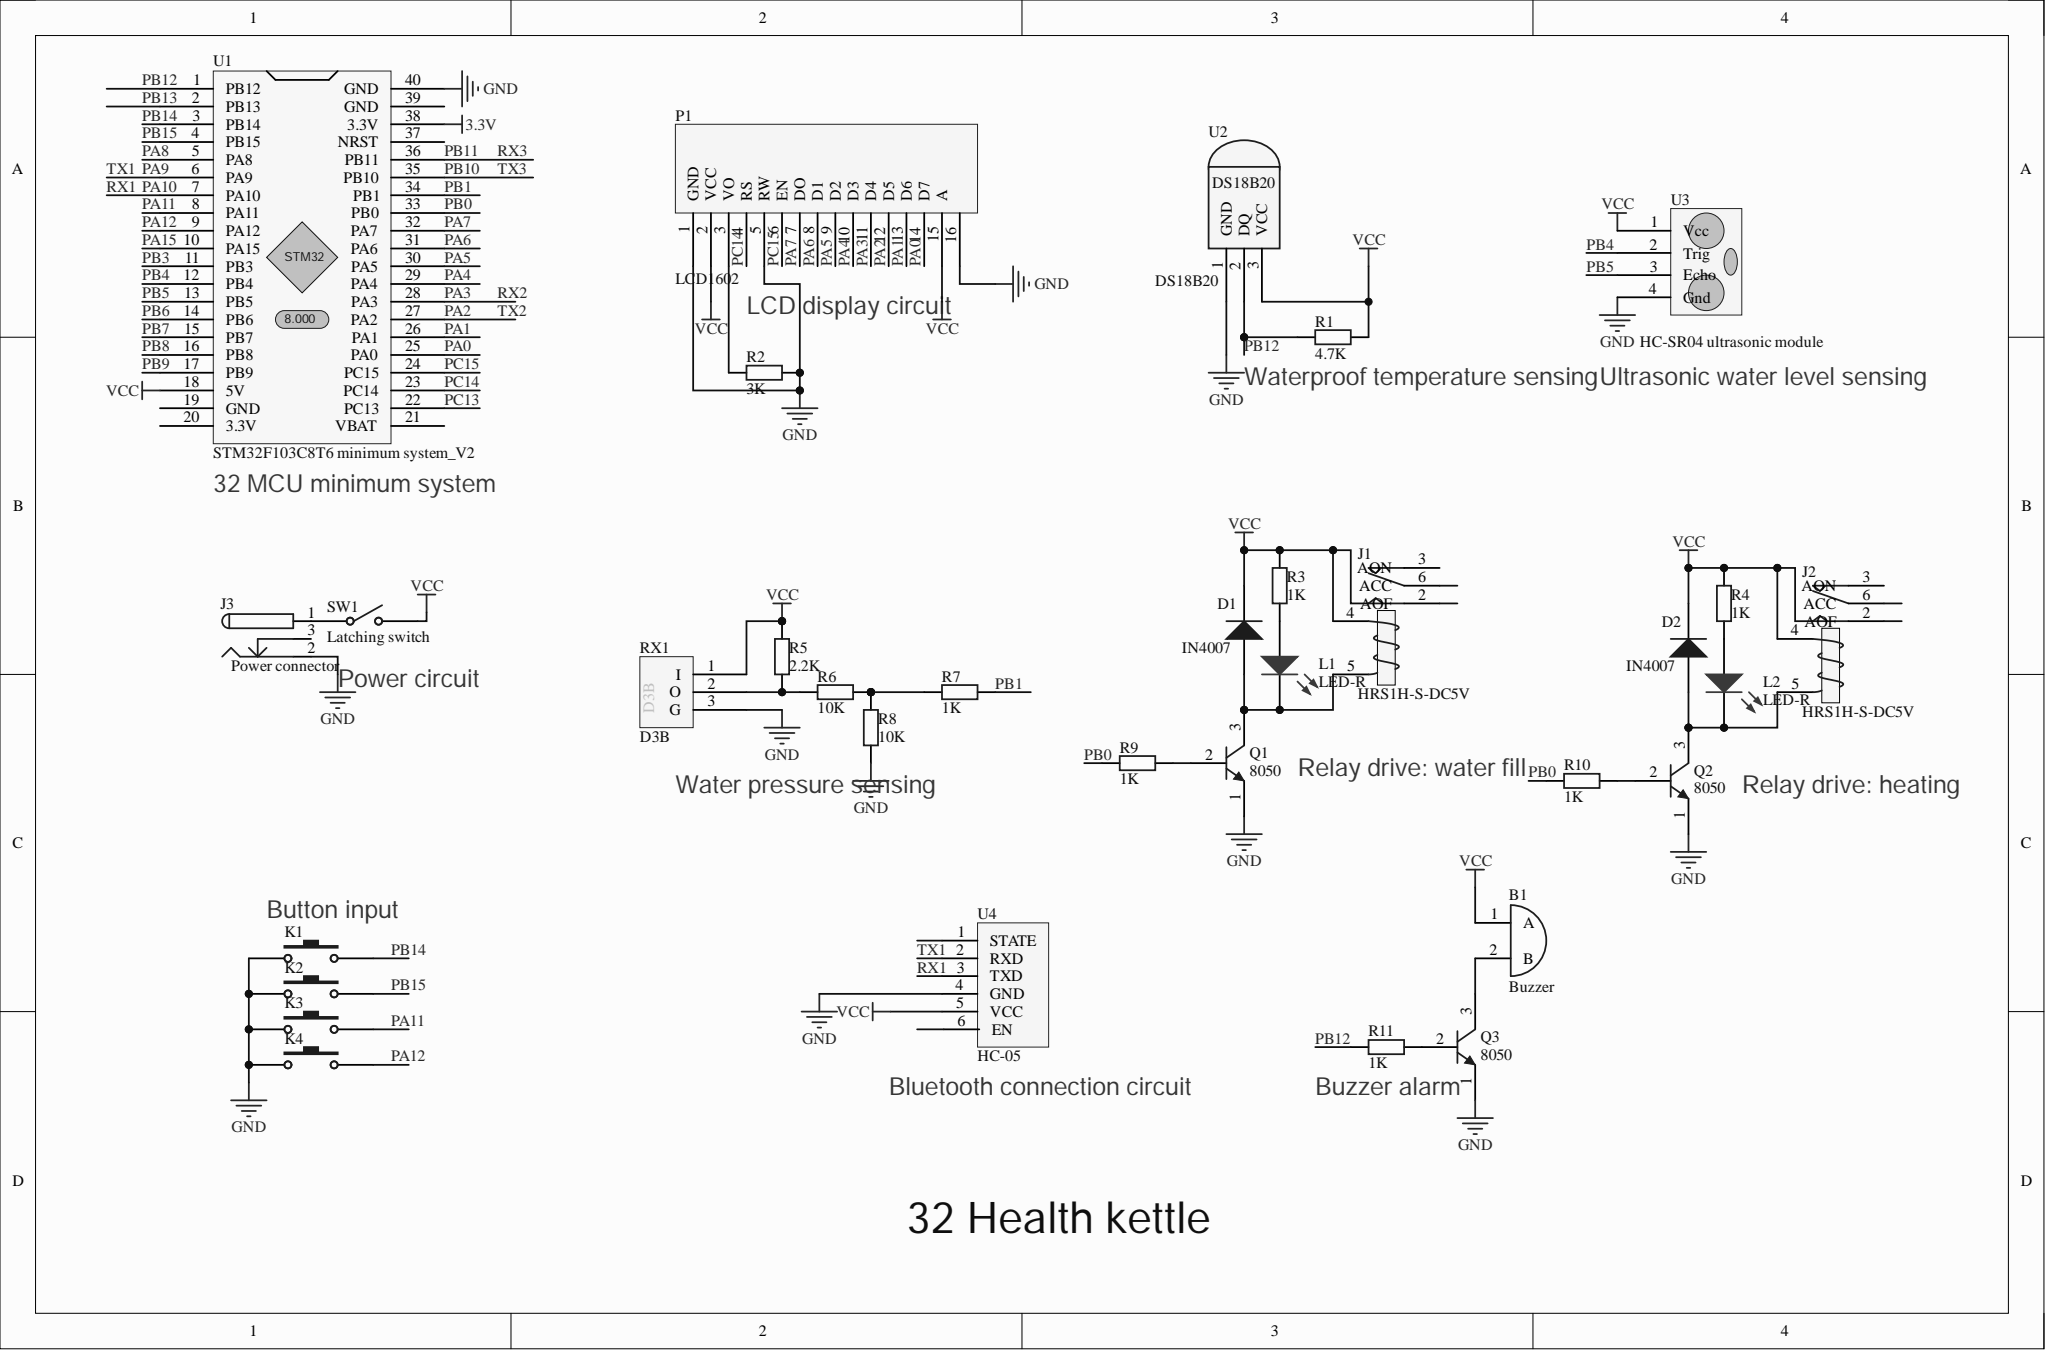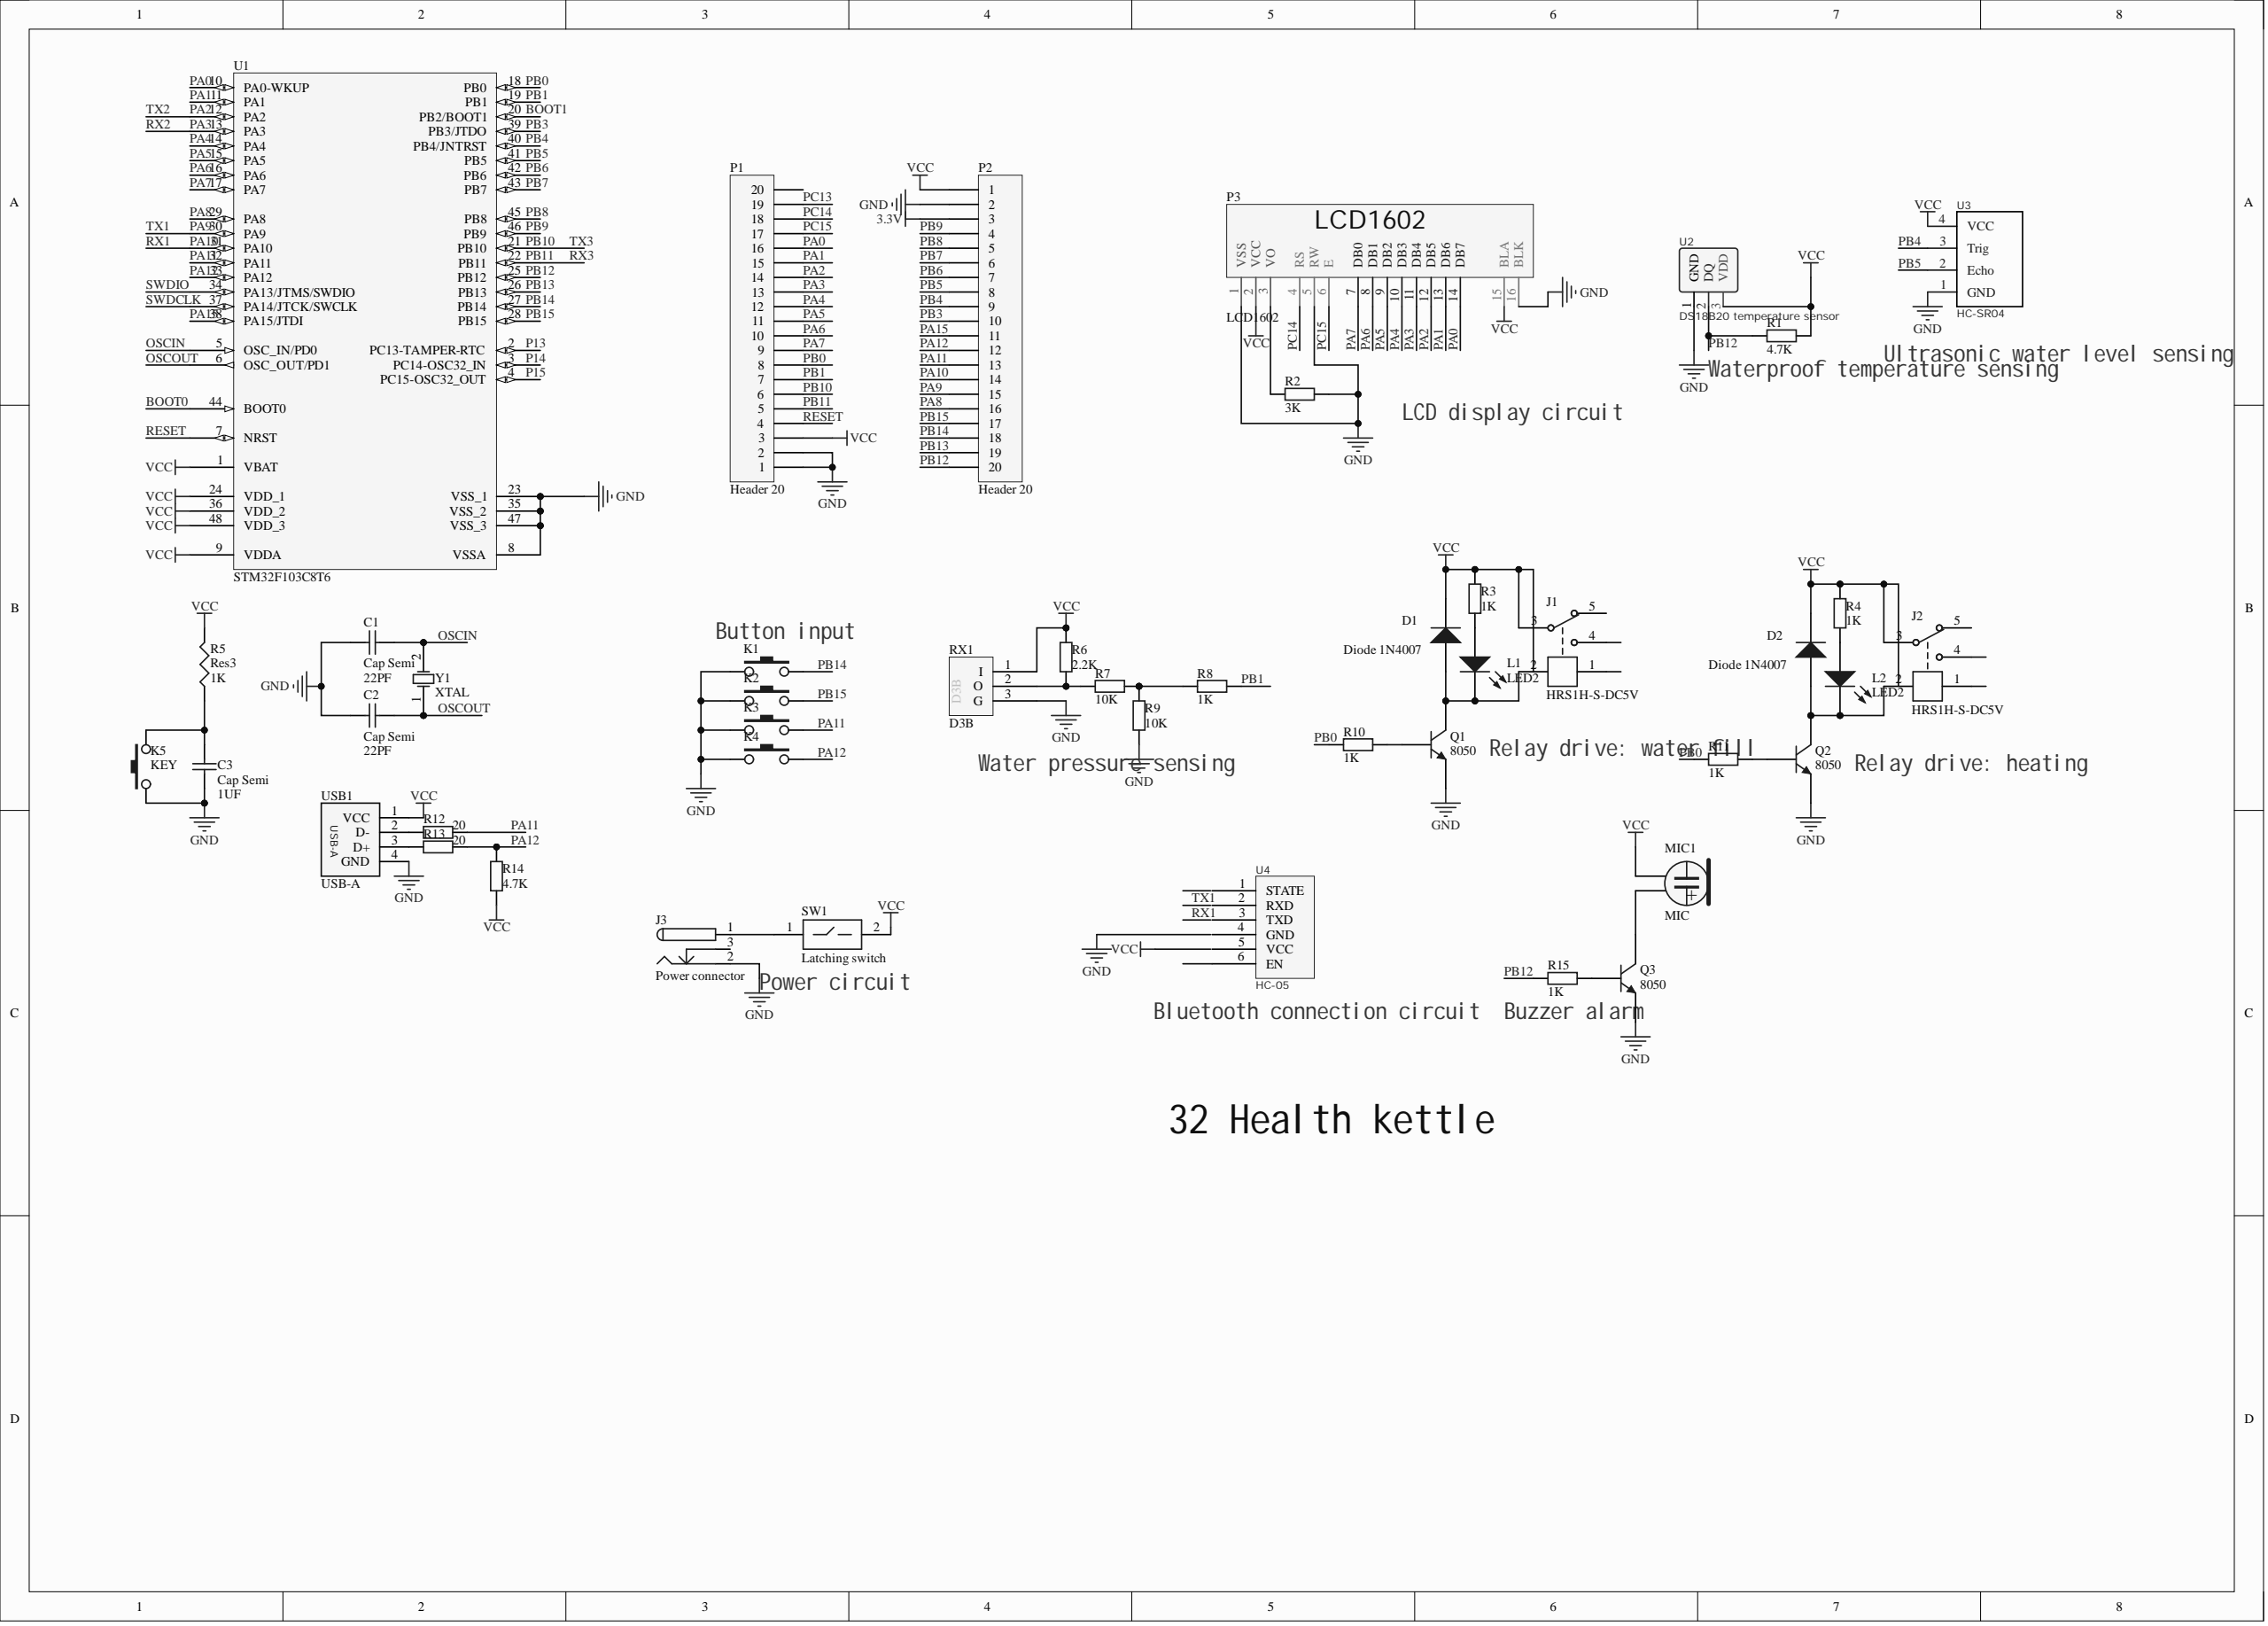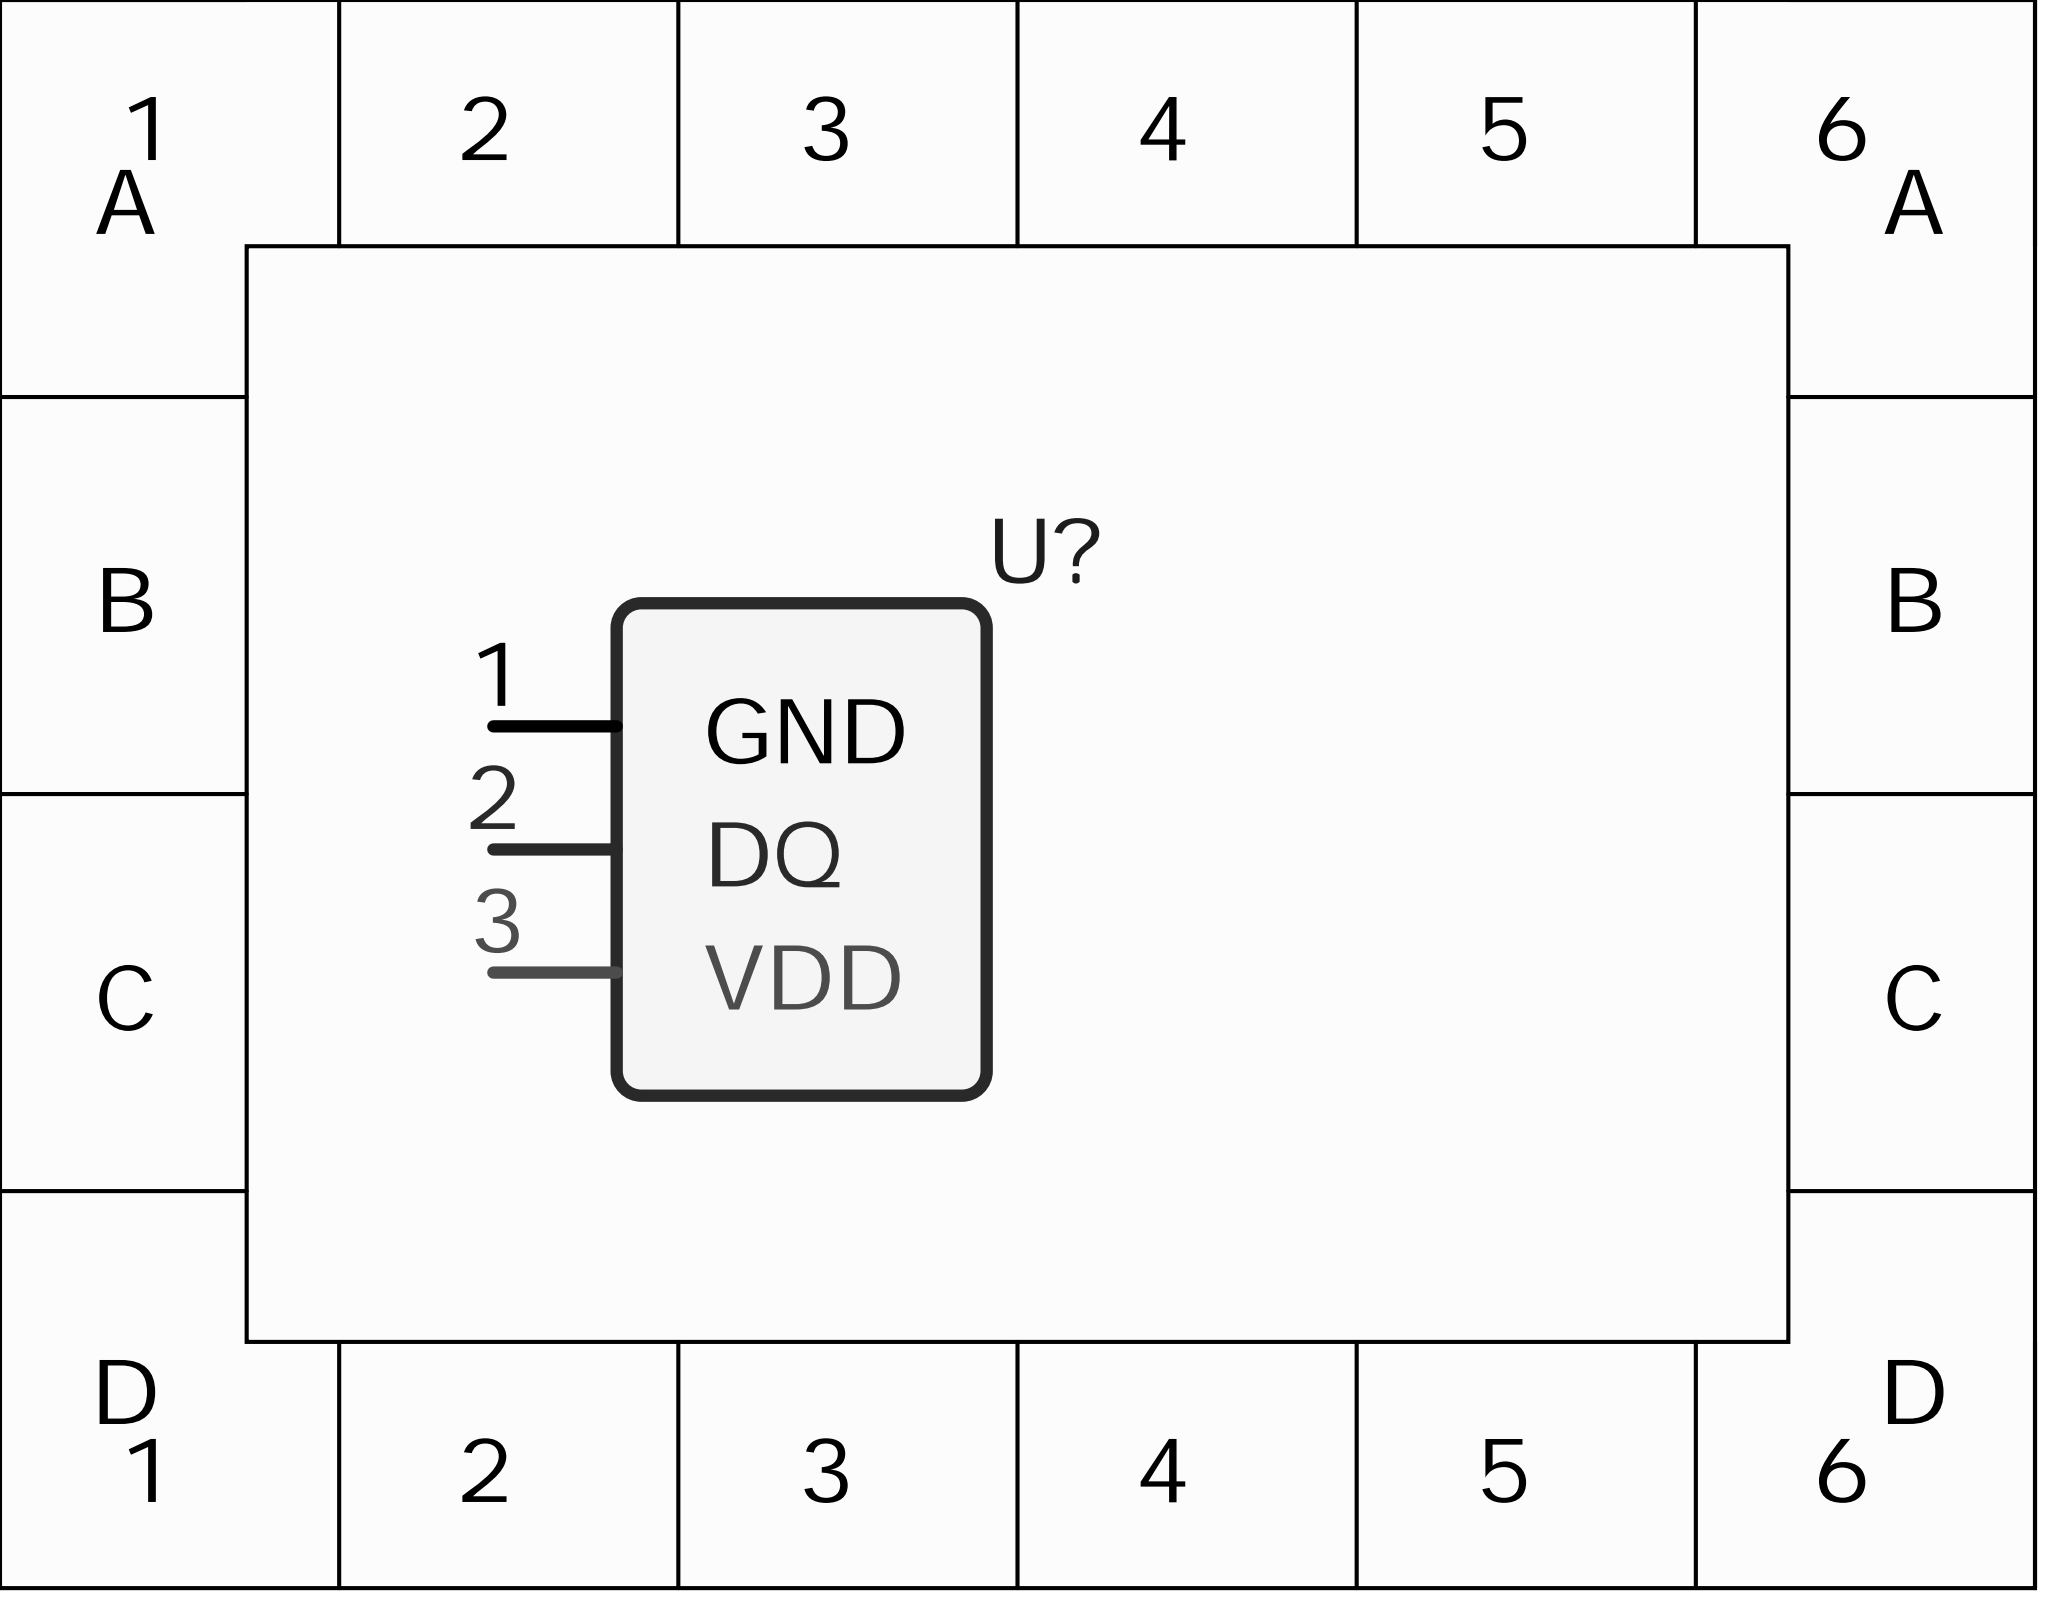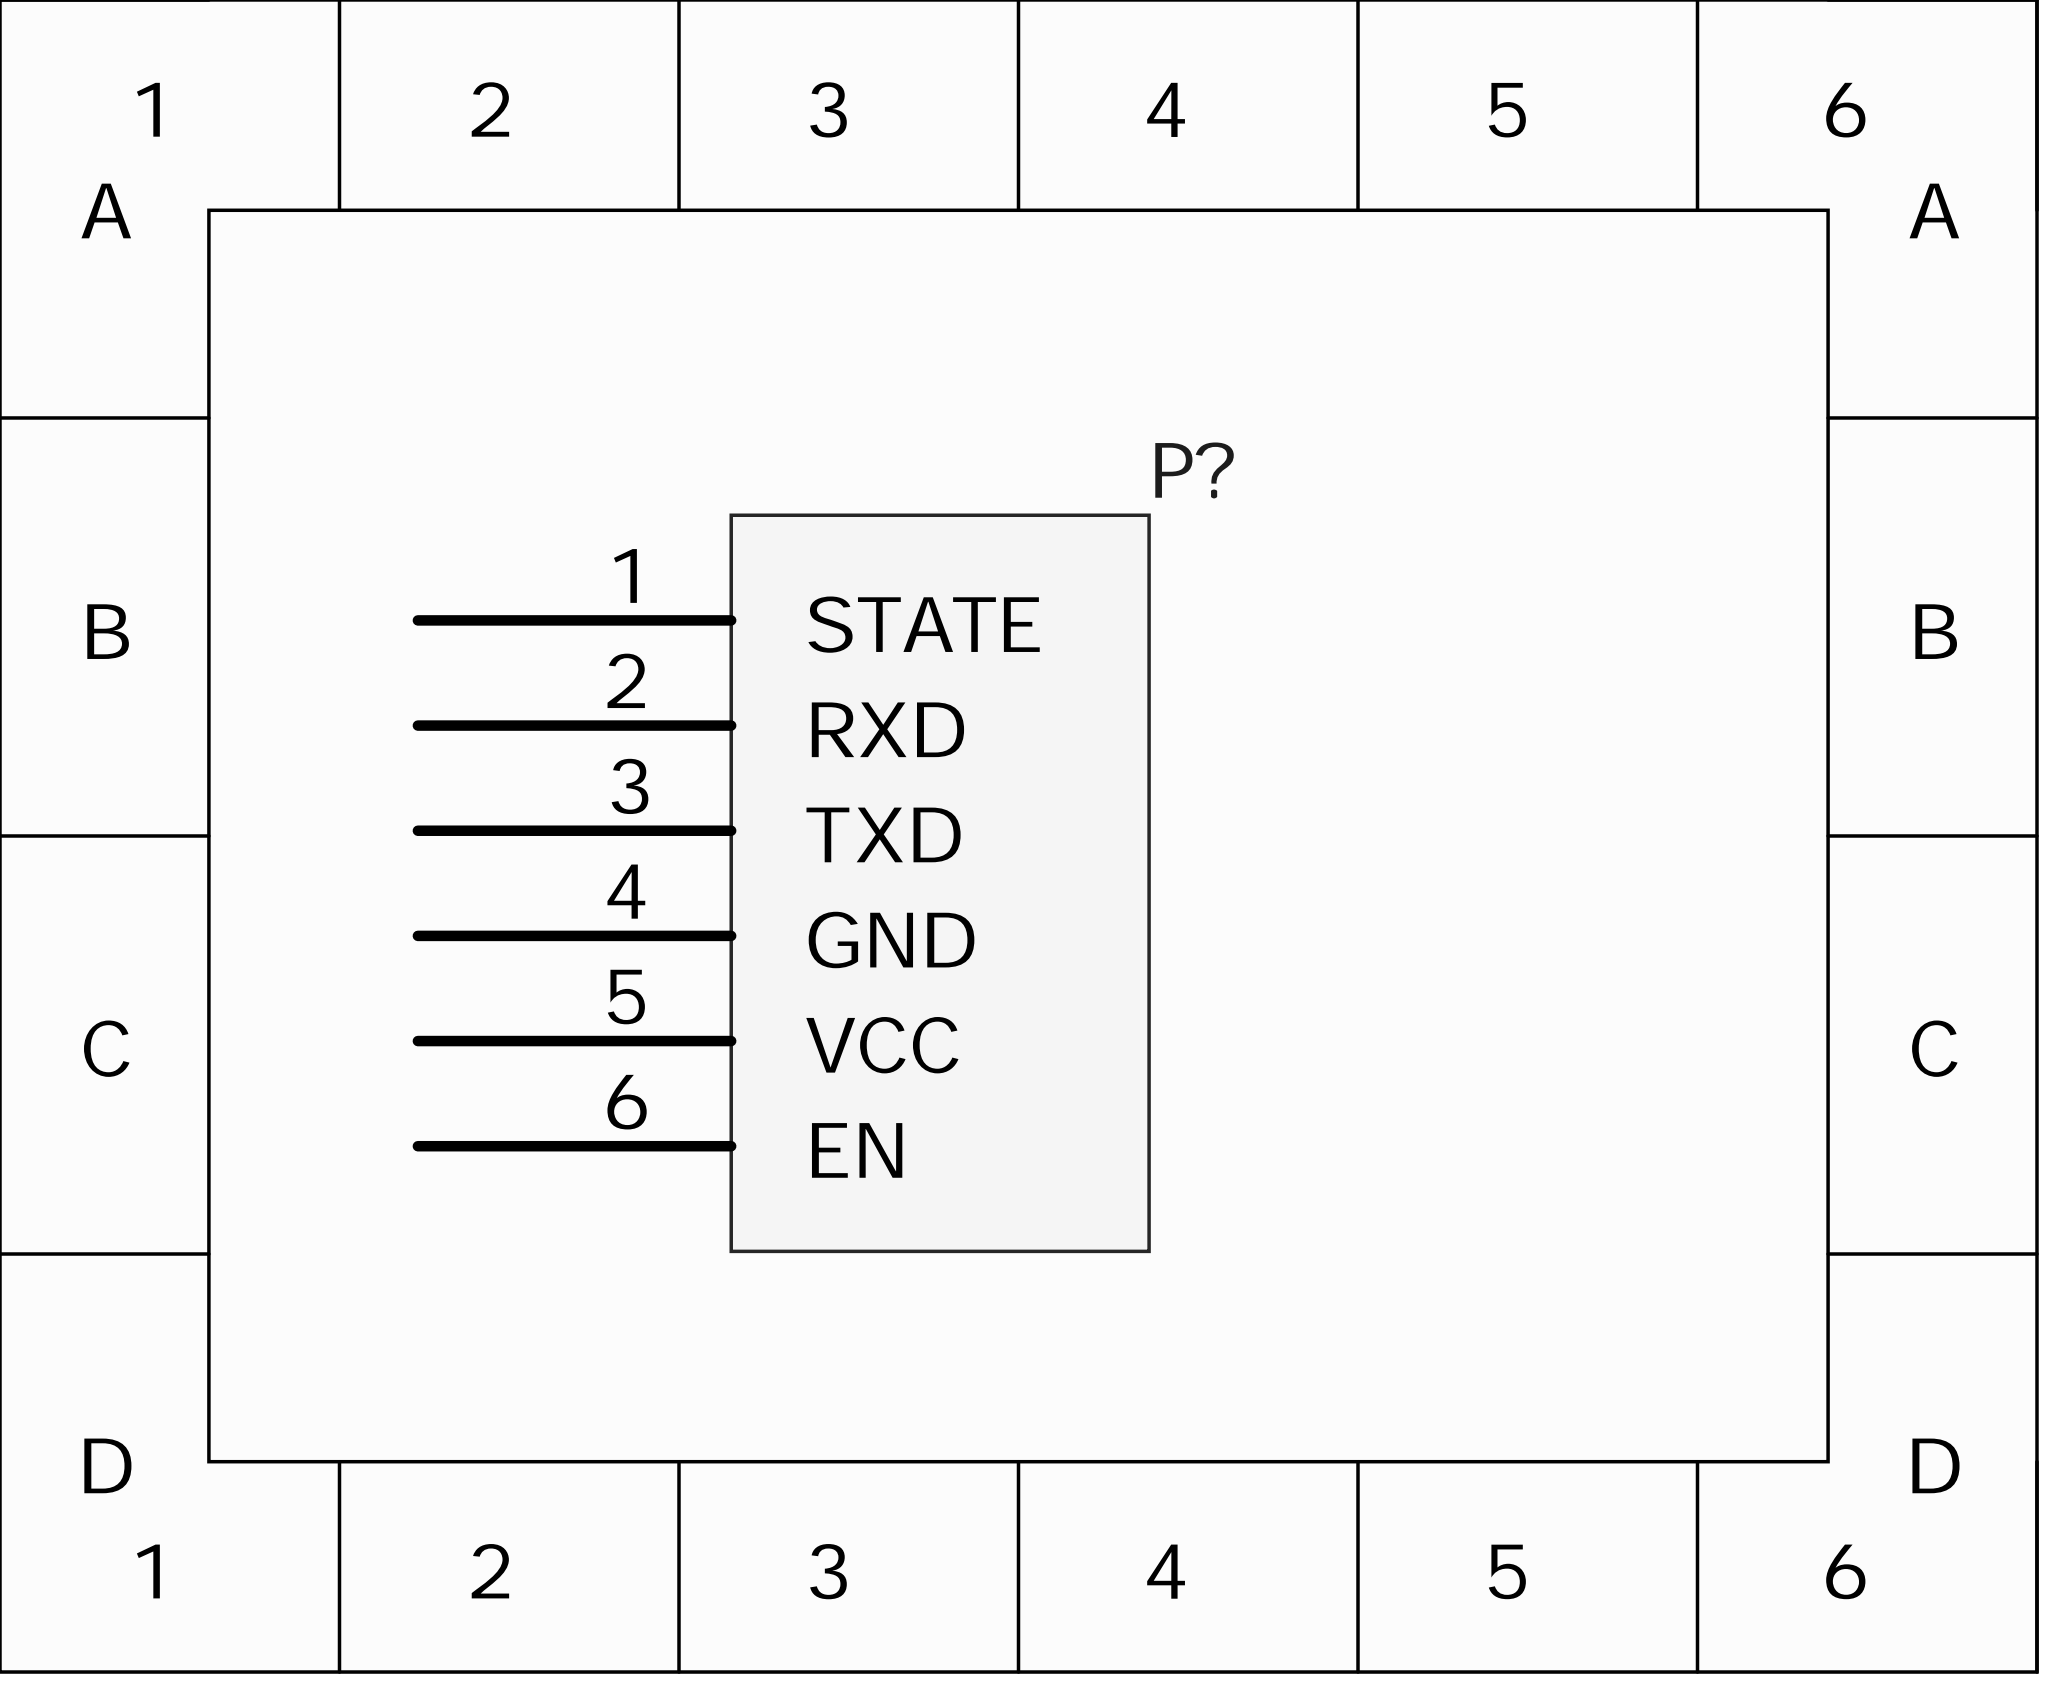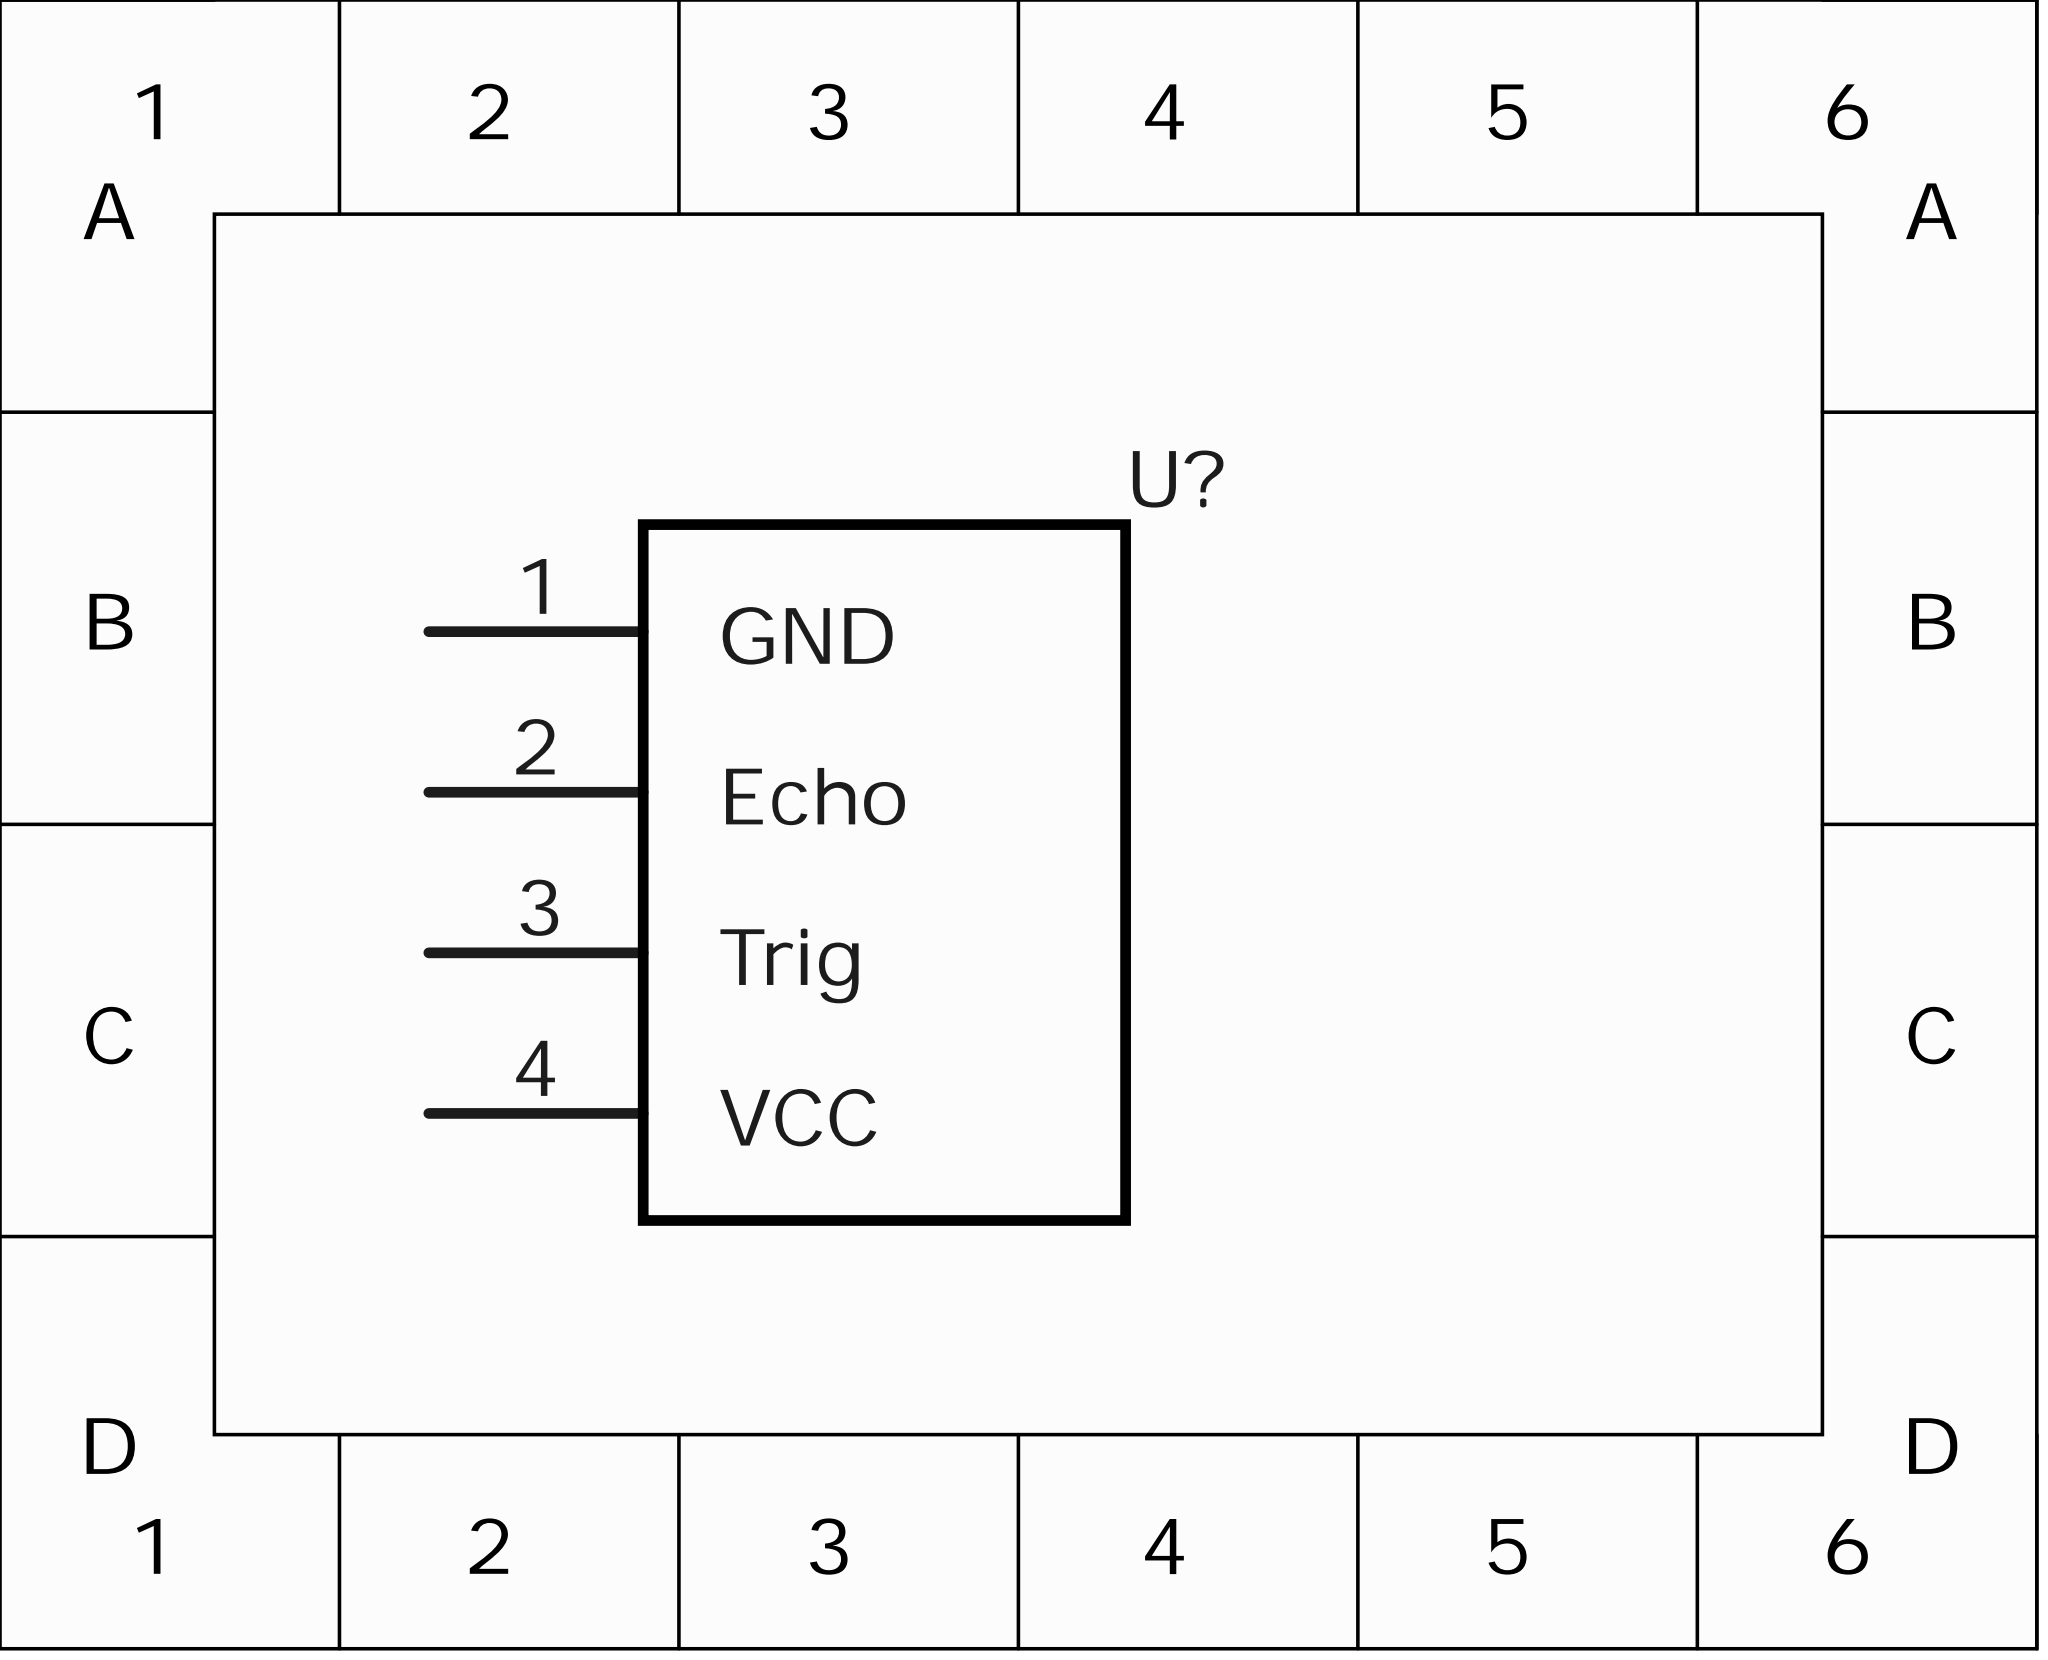Circuit board | Altium Designer | 81 parts | 65 nets
Bill of materials:
Comment,Description,Designator,Footprint,LibRef,Quantity
"Buzzer","Electrical Bell","B1","Buzzy-Small","Bell","1"
"Cap Semi","Capacitor (Semiconductor SIM Model)","C1, C2, C3","C1206","Cap Semi","3"
"Diode 1N4007","1 Amp General Purpose Rectifier","D1, D2","DO-41","Diode 1N4007","2"
"IN4007","","D1, D2","Diode-0.3","DIODE","2"
"HRS1H-S-DC5V","5V SPDT changeover","J1, J2","HRS1H","HRS1H-S-DC5V","2"
"HRS1H-S-DC5V","","J1, J2","JDIANQI","jidianqi","2"
"Power connector","","J3","DC-002","DC_Socket","1"
"Power connector","Low Voltage Power Supply Connector","J3","DC-JACK","DC002","1"
"Tactile button","","K1, K2, K3, K4","SW-6-6","SW-AJ","4"
"KEY","","K1, K2, K3, K4, K5","DIP-3X6X4.3","KEY","5"
"LED2","Typical RED, GREEN, YELLOW, AMBER GaAs LED","L1, L2","3.2X1.6X1.1","LED2","2"
"LED-R","","L1, L2","LED-3","LED-R","2"
"MIC","Condenser microphone","MIC1","MIC-4.5X1.9","MIC","1"
"LCD1602","","P1","1602","LCD1602","1"
"Header 20","Header, 20-Pin","P1, P2","HDR1X20","Header 20","2"
"LCD1602","","P3","LCD1602","LCD1602","1"
"","","P?","HC-05","HC-05","1"
"8050","","Q1, Q2, Q3","TO-92-2N3906","8050","3"
"8050","NPN Bipolar Transistor","Q1, Q2, Q3","TO-226-AA","NPN","3"
"4.7K","Resistor","R1, R14","AXIAL-0.3","RES2","3"
"3K","Resistor","R2","AXIAL-0.3","Res2","2"
"1K","Resistor, [NoValue]","R3, R4, R7, R8, R9, R10, R11, R15","AXIAL-0.3","Res2, RES0.4","12"
"Res3","Resistor","R5","J1-0603","Res3","1"
"2.2K","Resistor","R5, R6","AXIAL-0.3","RES2","2"
"10K","Resistor","R6, R7, R8, R9","AXIAL-0.3","RES2","4"
"20","Resistor","R12, R13","AXIAL-0.3","RES2","2"
"D3B","","RX1","HDR1X3","D3B","2"
"Latching switch","","SW1","DIP-1P","SW1-DIP2","1"
"Latching switch","","SW1","SW1","SW-SPST","1"
"STM32F103C8T6","STM32 ARM-based 32-bit MCU with 64 Kbytes Flash, 48-pin LQFP, Industrial Temperature","U1","LQFP48_N","STM32F103C8T6","1"
"STM32F103C8T6 minimum system_V2","","U1","STM32F103C8T6_V2","STM32F103C8T6最小系统_V2","1"
"DS18B20","","U2","DS18b20","DS18B20","1"
"DS18B20 temperature sensor","","U2","DS18B20温度传感器","DS18B20温度传感器","1"
"HC-SR04","HC","U3","HC-SR04","HC","1"
"HC-SR04 ultrasonic module","","U3","chaoshengbo-4","HC-SR04","1"
"HC-05","","U4","bluetooth","Bluetooth","1"
"HC-05","","U4","HC-05","HC-05","1"
"","","U?","DS18B20温度传感器","DS18B20温度传感器","1"
"","","U?","HC-SR04","HC-SR04","1"
"USB-A","","USB1","USB-A/S_A","USB-A","1"
"XTAL","Crystal Oscillator","Y1","R38","XTAL","1"
Netlist (Protel format):
[
B1
Buzzy-Small
Buzzer



]
[
C1
C1206
Cap Semi



]
[
C2
C1206
Cap Semi



]
[
C3
C1206
Cap Semi



]
[
D1
Diode-0.3
IN4007



]
[
D1
DO-41
Diode 1N4007



]
[
D2
Diode-0.3
IN4007



]
[
D2
DO-41
Diode 1N4007



]
[
J1
JDIANQI
HRS1H-S-DC5V



]
[
J1
HRS1H
HRS1H-S-DC5V



]
[
J2
JDIANQI
HRS1H-S-DC5V



]
[
J2
HRS1H
HRS1H-S-DC5V



]
[
J3
DC-JACK
Power connector



]
[
J3
DC-002
Power connector



]
[
K1
SW-6-6
Tactile button



]
[
K1
DIP-3X6X4.3
KEY



]
[
K2
SW-6-6
Tactile button



]
[
K2
DIP-3X6X4.3
KEY



]
[
K3
SW-6-6
Tactile button



]
[
K3
DIP-3X6X4.3
KEY



]
[
K4
SW-6-6
Tactile button



]
[
K4
DIP-3X6X4.3
KEY



]
[
K5
DIP-3X6X4.3
KEY



]
[
L1
LED-3
LED-R



]
[
L1
3.2X1.6X1.1
LED2



]
[
L2
LED-3
LED-R



]
[
L2
3.2X1.6X1.1
LED2



]
[
MIC1
MIC-4.5X1.9
MIC



]
[
P1
1602
LCD1602



]
[
P1
HDR1X20
Header 20



]
[
P2
HDR1X20
Header 20



]
[
P3
LCD1602
LCD1602



]
[
P?
HC-05




]
[
Q1
TO-92-2N3906
8050



]
[
Q1
TO-226-AA
8050



]
[
Q2
TO-92-2N3906
8050



]
[
Q2
TO-226-AA
8050



]
[
Q3
TO-92-2N3906
8050



]
[
Q3
TO-226-AA
8050



]
[
R1
AXIAL-0.3
4.7K



]
[
R1
AXIAL-0.3
4.7K



]
[
R2
AXIAL-0.3
3K



]
[
R2
AXIAL-0.3
3K



]
[
R3
AXIAL-0.3
1K



]
[
R3
AXIAL-0.3
1K



]
[
R4
AXIAL-0.3
1K



]
[
R4
AXIAL-0.3
1K



]
[
R5
AXIAL-0.3
2.2K



]
[
R5
J1-0603
Res3



]
[
R6
AXIAL-0.3
10K



]
[
R6
AXIAL-0.3
2.2K



]
[
R7
AXIAL-0.3
1K



]
[
R7
AXIAL-0.3
10K



]
[
R8
AXIAL-0.3
10K



]
[
R8
AXIAL-0.3
1K



]
[
R9
AXIAL-0.3
1K



]
[
R9
AXIAL-0.3
10K



]
[
R10
AXIAL-0.3
1K



]
[
R10
AXIAL-0.3
1K



]
[
R11
AXIAL-0.3
1K



]
[
R11
AXIAL-0.3
1K



]
[
R12
AXIAL-0.3
20



]
[
R13
AXIAL-0.3
20



]
[
R14
AXIAL-0.3
4.7K



]
[
R15
AXIAL-0.3
1K



]
[
RX1
HDR1X3
D3B



]
[
RX1
HDR1X3
D3B



]
[
SW1
SW1
Latching switch



]
[
SW1
DIP-1P
Latching switch



]
[
U1
STM32F103C8T6_V2
STM32F103C8T6 minimum system_V2



]
[
U1
LQFP48_N
STM32F103C8T6



]
[
U2
DS18b20
DS18B20



]
[
U2
DS18B20温度传感器
DS18B20 temperature sensor



]
[
U3
chaoshengbo-4
HC-SR04 ultrasonic module



]
[
U3
HC-SR04
HC-SR04



]
[
U4
bluetooth
HC-05



]
[
U4
HC-05
HC-05



]
[
U?
DS18B20温度传感器




]
[
U?
HC-SR04




]
[
USB1
USB-A/S_A
USB-A



]
[
Y1
R38
XTAL



]
(
VCC
B1-1
D1-2
D1-2
D2-2
D2-2
J1-3
J1-4
J2-3
J2-4
MIC1-2
P1-2
P1-3
P1-15
P2-1
P3-2
P3-15
R1-2
R1-2
R3-2
R3-2
R4-2
R4-2
R5-2
R5-2
R6-2
R14-2
RX1-1
RX1-1
SW1-2
SW1-2
U1-1
U1-9
U1-18
U1-24
U1-36
U1-48
U2-3
U2-3
U3-1
U3-4
U4-5
USB1-1
)
(
RESET
P1-4
U1-7
)
(
PC15
P1-6
P1-17
P3-6
U1-24
)
(
PC14
P1-4
P1-18
P3-4
U1-23
)
(
PC13
P1-19
U1-22
)
(
PB15
K2-2
K2-3
P2-17
U1-4
)
(
PB14
K1-2
K1-3
P2-18
U1-3
)
(
PB13
P2-19
U1-2
)
(
PB12
P2-20
R1-1
R1-1
R11-1
R15-1
U1-1
U2-2
U2-2
)
(
PB11
P1-5
U1-22
U1-36
)
(
PB10
P1-6
U1-21
U1-35
)
(
PB9
P2-4
U1-17
)
(
PB8
P2-5
U1-16
)
(
PB7
P2-6
U1-15
)
(
PB6
P2-7
U1-14
)
(
PB5
P2-8
U1-13
U3-2
U3-3
)
(
PB4
P2-9
U1-12
U3-2
U3-3
)
(
PB3
P2-10
U1-11
)
(
PB1
P1-7
R7-1
R8-1
U1-34
)
(
PB0
P1-8
R9-1
R10-1
R10-1
R11-1
U1-33
)
(
PA15
P2-11
U1-10
U1-38
)
(
PA12
K4-2
K4-3
P2-12
R13-1
R14-1
U1-9
U1-33
)
(
PA11
K3-2
K3-3
P2-13
R12-1
U1-8
U1-32
)
(
PA10
P2-14
U1-7
U1-31
U4-3
)
(
PA9
P2-15
U1-6
U1-30
U4-2
)
(
PA8
P2-16
U1-5
U1-29
)
(
PA7
P1-7
P1-9
P3-7
U1-17
U1-32
)
(
PA6
P1-8
P1-10
P3-8
U1-16
U1-31
)
(
PA5
P1-9
P1-11
P3-9
U1-15
U1-30
)
(
PA4
P1-10
P1-12
P3-10
U1-14
U1-29
)
(
PA3
P1-11
P1-13
P3-11
U1-13
U1-28
)
(
PA2
P1-12
P1-14
P3-12
U1-12
U1-27
)
(
PA1
P1-13
P1-15
P3-13
U1-11
U1-26
)
(
PA0
P1-14
P1-16
P3-14
U1-10
U1-25
)
(
OSCOUT
C2-1
U1-6
Y1-1
)
(
OSCIN
C1-1
U1-5
Y1-2
)
(
NetR13_2
R13-2
USB1-3
)
(
NetR12_2
R12-2
USB1-2
)
(
NetR7_2
R7-2
R8-2
R9-2
)
(
NetR6_2
R6-2
R7-2
R8-2
)
(
NetR6_1
R6-1
R7-1
RX1-2
)
(
NetR5_1
R5-1
R6-1
RX1-2
)
(
NetQ3_2
Q3-2
R11-2
)
(
NetQ3_2
Q3-2
R15-2
)
(
NetQ2_2
Q2-2
R10-2
)
(
NetQ2_2
Q2-2
R11-2
)
(
NetQ1_2
Q1-2
R9-2
)
(
NetQ1_2
Q1-2
R10-2
)
(
NetP3_3
P3-3
R2-1
)
(
NetP1_3
P1-3
R2-1
)
(
NetMIC1_1
MIC1-1
Q3-1
)
(
NetL2_1
L2-1
R4-1
)
(
NetL2_1
L2-1
R4-1
)
(
NetL1_1
L1-1
R3-1
)
(
NetL1_1
L1-1
R3-1
)
(
NetJ3_1
J3-1
SW1-1
)
(
NetJ3_1
J3-1
SW1-1
)
(
NetD2_1
D2-1
J2-5
L2-2
Q2-3
)
(
NetD2_1
D2-1
J2-2
L2-2
Q2-1
)
(
NetD1_1
D1-1
J1-5
L1-2
Q1-3
)
(
NetD1_1
D1-1
J1-2
L1-2
Q1-1
)
(
NetC3_2
C3-2
K5-3
R5-1
)
(
NetB1_2
B1-2
Q3-3
)
(
GND
C1-2
C2-2
C3-1
J3-2
J3-2
K1-1
K1-1
K2-1
K2-1
K3-1
K3-1
K4-1
K4-1
K5-1
P1-1
P1-1
P1-2
P1-5
P1-16
P2-2
P3-1
P3-5
P3-16
Q1-1
Q1-3
Q2-1
Q2-3
Q3-1
Q3-3
R2-2
R2-2
R8-1
R9-1
RX1-3
RX1-3
U1-8
U1-23
U1-35
U1-40
U1-47
U2-1
U2-1
U3-1
U3-4
U4-4
USB1-4
)
(
3.3V
P2-3
U1-38
)